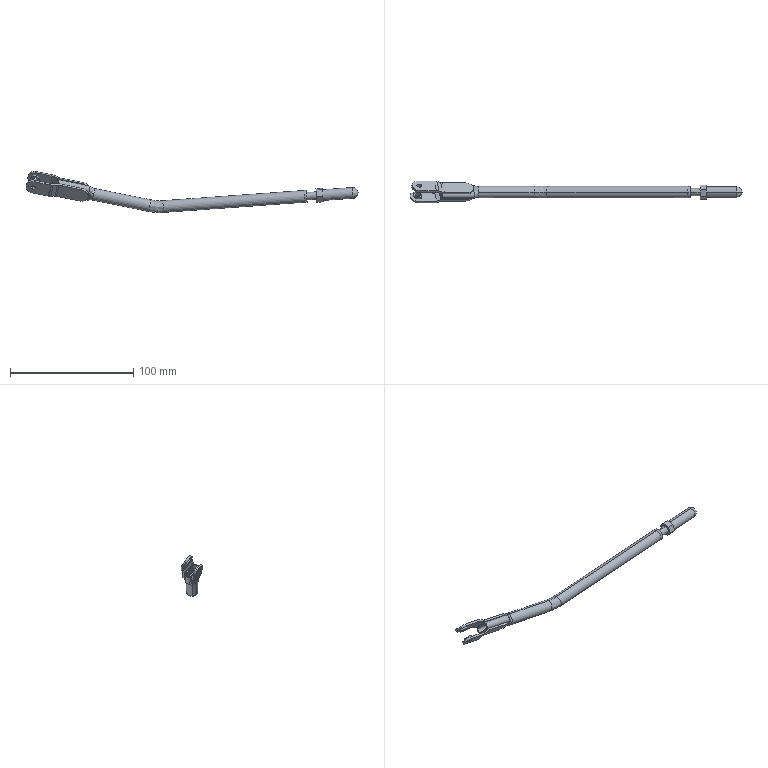Part | SolidWorks | features BaseBody 8 | 8 solids | 96 faces | box 269.089 x 17.657 x 33.299 mm | volume 8974 mm3 | cylinder 48 | plane 40 | spline 6 | torus 2 | commonest cylinder face diameters 4.2 x8 9.5 x6 12 x6 10 x5 6.797 x4 7.9 x4